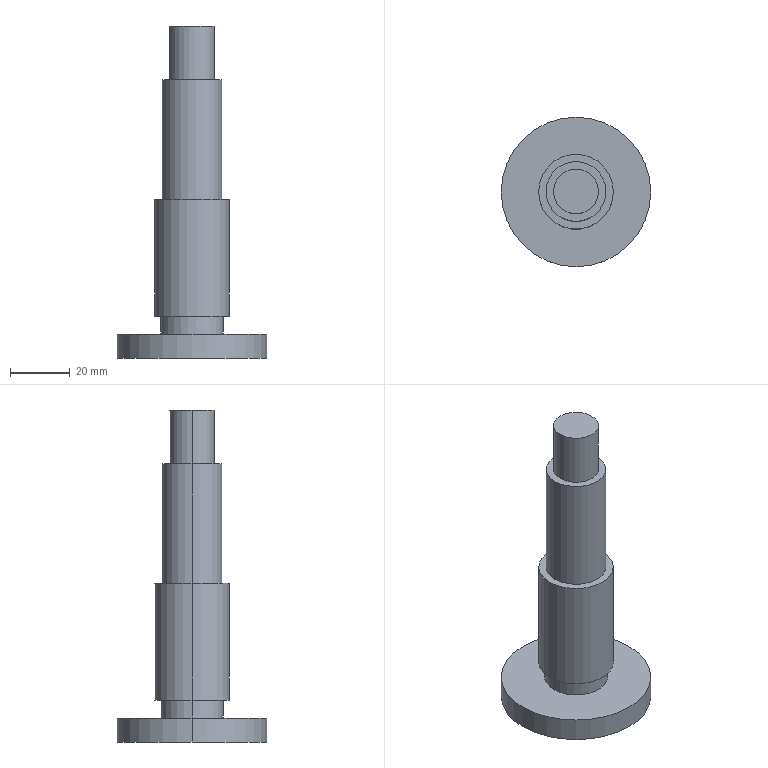Part | SolidWorks | features ICE 3, Extrusion 1, RevCut 1 | 1 solid | 16 faces | box 50 x 50 x 111 mm | volume 52677 mm3 | cylinder 10 | plane 6 | commonest cylinder face diameters 15 x2 20 x2 21 x2 25 x2 50 x2
STEP:
#1=CARTESIAN_POINT('',(7.5,0.,103.));
#2=VERTEX_POINT('',#1);
#3=CARTESIAN_POINT('',(-7.5,0.,103.));
#4=VERTEX_POINT('',#3);
#5=CARTESIAN_POINT('',(0.,0.,103.));
#6=DIRECTION('',(0.,0.,1.));
#7=DIRECTION('',(1.,0.,0.));
#8=AXIS2_PLACEMENT_3D('',#5,#6,#7);
#9=CIRCLE('',#8,7.5);
#10=EDGE_CURVE('',#2,#4,#9,.T.);
#11=ORIENTED_EDGE('',*,*,#10,.F.);
#12=CARTESIAN_POINT('',(7.5,0.,85.));
#13=VERTEX_POINT('',#12);
#14=CARTESIAN_POINT('',(7.5,0.,103.));
#15=DIRECTION('',(0.,0.,-1.));
#16=VECTOR('',#15,1000.);
#17=LINE('',#14,#16);
#18=EDGE_CURVE('',#2,#13,#17,.T.);
#19=ORIENTED_EDGE('',*,*,#18,.T.);
#20=CARTESIAN_POINT('',(-7.5,0.,85.));
#21=VERTEX_POINT('',#20);
#22=CARTESIAN_POINT('',(0.,0.,85.));
#23=DIRECTION('',(0.,0.,1.));
#24=DIRECTION('',(1.,0.,0.));
#25=AXIS2_PLACEMENT_3D('',#22,#23,#24);
#26=CIRCLE('',#25,7.5);
#27=EDGE_CURVE('',#13,#21,#26,.T.);
#28=ORIENTED_EDGE('',*,*,#27,.T.);
#29=CARTESIAN_POINT('',(-7.5,0.,103.));
#30=DIRECTION('',(0.,0.,-1.));
#31=VECTOR('',#30,1000.);
#32=LINE('',#29,#31);
#33=EDGE_CURVE('',#4,#21,#32,.T.);
#34=ORIENTED_EDGE('',*,*,#33,.F.);
#35=EDGE_LOOP('',(#11,#19,#28,#34));
#36=FACE_OUTER_BOUND('',#35,.T.);
#37=CARTESIAN_POINT('',(0.,0.,103.));
#38=DIRECTION('',(0.,0.,-1.));
#39=DIRECTION('',(-1.,0.,0.));
#40=AXIS2_PLACEMENT_3D('',#37,#38,#39);
#41=CYLINDRICAL_SURFACE('',#40,7.5);
#42=ADVANCED_FACE('',(#36),#41,.T.);
#43=CARTESIAN_POINT('',(-25.,0.,-8.));
#44=VERTEX_POINT('',#43);
#45=CARTESIAN_POINT('',(25.,0.,-8.));
#46=VERTEX_POINT('',#45);
#47=CARTESIAN_POINT('',(0.,0.,-8.));
#48=DIRECTION('',(0.,0.,-1.));
#49=DIRECTION('',(-1.,0.,0.));
#50=AXIS2_PLACEMENT_3D('',#47,#48,#49);
#51=CIRCLE('',#50,25.);
#52=EDGE_CURVE('',#44,#46,#51,.T.);
#53=ORIENTED_EDGE('',*,*,#52,.F.);
#54=CARTESIAN_POINT('',(-25.,0.,0.));
#55=VERTEX_POINT('',#54);
#56=CARTESIAN_POINT('',(-25.,0.,-8.));
#57=DIRECTION('',(0.,0.,1.));
#58=VECTOR('',#57,1000.);
#59=LINE('',#56,#58);
#60=EDGE_CURVE('',#44,#55,#59,.T.);
#61=ORIENTED_EDGE('',*,*,#60,.T.);
#62=CARTESIAN_POINT('',(25.,0.,0.));
#63=VERTEX_POINT('',#62);
#64=CARTESIAN_POINT('',(0.,0.,0.));
#65=DIRECTION('',(0.,0.,-1.));
#66=DIRECTION('',(-1.,0.,0.));
#67=AXIS2_PLACEMENT_3D('',#64,#65,#66);
#68=CIRCLE('',#67,25.);
#69=EDGE_CURVE('',#55,#63,#68,.T.);
#70=ORIENTED_EDGE('',*,*,#69,.T.);
#71=CARTESIAN_POINT('',(25.,0.,-8.));
#72=DIRECTION('',(0.,0.,1.));
#73=VECTOR('',#72,1000.);
#74=LINE('',#71,#73);
#75=EDGE_CURVE('',#46,#63,#74,.T.);
#76=ORIENTED_EDGE('',*,*,#75,.F.);
#77=EDGE_LOOP('',(#53,#61,#70,#76));
#78=FACE_OUTER_BOUND('',#77,.T.);
#79=CARTESIAN_POINT('',(0.,0.,-8.));
#80=DIRECTION('',(0.,0.,1.));
#81=DIRECTION('',(1.,0.,0.));
#82=AXIS2_PLACEMENT_3D('',#79,#80,#81);
#83=CYLINDRICAL_SURFACE('',#82,25.);
#84=ADVANCED_FACE('',(#78),#83,.T.);
#85=CARTESIAN_POINT('',(-10.5,0.,6.));
#86=VERTEX_POINT('',#85);
#87=CARTESIAN_POINT('',(10.5,0.,6.));
#88=VERTEX_POINT('',#87);
#89=CARTESIAN_POINT('',(0.,0.,6.));
#90=DIRECTION('',(0.,0.,-1.));
#91=DIRECTION('',(-1.,0.,0.));
#92=AXIS2_PLACEMENT_3D('',#89,#90,#91);
#93=CIRCLE('',#92,10.5);
#94=EDGE_CURVE('',#86,#88,#93,.T.);
#95=ORIENTED_EDGE('',*,*,#94,.T.);
#96=CARTESIAN_POINT('',(10.5,0.,0.));
#97=VERTEX_POINT('',#96);
#98=CARTESIAN_POINT('',(10.5,0.,0.));
#99=DIRECTION('',(0.,0.,-1.));
#100=VECTOR('',#99,1000.);
#101=LINE('',#98,#100);
#102=EDGE_CURVE('',#88,#97,#101,.T.);
#103=ORIENTED_EDGE('',*,*,#102,.T.);
#104=CARTESIAN_POINT('',(-10.5,0.,0.));
#105=VERTEX_POINT('',#104);
#106=CARTESIAN_POINT('',(0.,0.,0.));
#107=DIRECTION('',(0.,0.,-1.));
#108=DIRECTION('',(-1.,0.,0.));
#109=AXIS2_PLACEMENT_3D('',#106,#107,#108);
#110=CIRCLE('',#109,10.5);
#111=EDGE_CURVE('',#105,#97,#110,.T.);
#112=ORIENTED_EDGE('',*,*,#111,.F.);
#113=CARTESIAN_POINT('',(-10.5,0.,0.));
#114=DIRECTION('',(0.,0.,-1.));
#115=VECTOR('',#114,1000.);
#116=LINE('',#113,#115);
#117=EDGE_CURVE('',#86,#105,#116,.T.);
#118=ORIENTED_EDGE('',*,*,#117,.F.);
#119=EDGE_LOOP('',(#95,#103,#112,#118));
#120=FACE_OUTER_BOUND('',#119,.T.);
#121=CARTESIAN_POINT('',(0.,0.,0.));
#122=DIRECTION('',(0.,0.,-1.));
#123=DIRECTION('',(-1.,0.,0.));
#124=AXIS2_PLACEMENT_3D('',#121,#122,#123);
#125=CYLINDRICAL_SURFACE('',#124,10.5);
#126=ADVANCED_FACE('',(#120),#125,.T.);
#127=CARTESIAN_POINT('',(10.,0.,85.));
#128=VERTEX_POINT('',#127);
#129=CARTESIAN_POINT('',(-10.,0.,85.));
#130=VERTEX_POINT('',#129);
#131=CARTESIAN_POINT('',(0.,0.,85.));
#132=DIRECTION('',(0.,0.,1.));
#133=DIRECTION('',(1.,0.,0.));
#134=AXIS2_PLACEMENT_3D('',#131,#132,#133);
#135=CIRCLE('',#134,10.);
#136=EDGE_CURVE('',#128,#130,#135,.T.);
#137=ORIENTED_EDGE('',*,*,#136,.F.);
#138=CARTESIAN_POINT('',(10.,0.,45.));
#139=VERTEX_POINT('',#138);
#140=CARTESIAN_POINT('',(10.,0.,85.));
#141=DIRECTION('',(0.,0.,-1.));
#142=VECTOR('',#141,1000.);
#143=LINE('',#140,#142);
#144=EDGE_CURVE('',#128,#139,#143,.T.);
#145=ORIENTED_EDGE('',*,*,#144,.T.);
#146=CARTESIAN_POINT('',(-10.,0.,45.));
#147=VERTEX_POINT('',#146);
#148=CARTESIAN_POINT('',(0.,0.,45.));
#149=DIRECTION('',(0.,0.,1.));
#150=DIRECTION('',(1.,0.,0.));
#151=AXIS2_PLACEMENT_3D('',#148,#149,#150);
#152=CIRCLE('',#151,10.);
#153=EDGE_CURVE('',#139,#147,#152,.T.);
#154=ORIENTED_EDGE('',*,*,#153,.T.);
#155=CARTESIAN_POINT('',(-10.,0.,85.));
#156=DIRECTION('',(0.,0.,-1.));
#157=VECTOR('',#156,1000.);
#158=LINE('',#155,#157);
#159=EDGE_CURVE('',#130,#147,#158,.T.);
#160=ORIENTED_EDGE('',*,*,#159,.F.);
#161=EDGE_LOOP('',(#137,#145,#154,#160));
#162=FACE_OUTER_BOUND('',#161,.T.);
#163=CARTESIAN_POINT('',(0.,0.,85.));
#164=DIRECTION('',(0.,0.,-1.));
#165=DIRECTION('',(-1.,0.,0.));
#166=AXIS2_PLACEMENT_3D('',#163,#164,#165);
#167=CYLINDRICAL_SURFACE('',#166,10.);
#168=ADVANCED_FACE('',(#162),#167,.T.);
#169=CARTESIAN_POINT('',(12.5,0.,45.));
#170=VERTEX_POINT('',#169);
#171=CARTESIAN_POINT('',(-12.5,0.,45.));
#172=VERTEX_POINT('',#171);
#173=CARTESIAN_POINT('',(0.,0.,45.));
#174=DIRECTION('',(0.,0.,1.));
#175=DIRECTION('',(1.,0.,0.));
#176=AXIS2_PLACEMENT_3D('',#173,#174,#175);
#177=CIRCLE('',#176,12.5);
#178=EDGE_CURVE('',#170,#172,#177,.T.);
#179=ORIENTED_EDGE('',*,*,#178,.F.);
#180=CARTESIAN_POINT('',(12.5,0.,6.));
#181=VERTEX_POINT('',#180);
#182=CARTESIAN_POINT('',(12.5,0.,45.));
#183=DIRECTION('',(0.,0.,-1.));
#184=VECTOR('',#183,1000.);
#185=LINE('',#182,#184);
#186=EDGE_CURVE('',#170,#181,#185,.T.);
#187=ORIENTED_EDGE('',*,*,#186,.T.);
#188=CARTESIAN_POINT('',(-12.5,0.,6.));
#189=VERTEX_POINT('',#188);
#190=CARTESIAN_POINT('',(0.,0.,6.));
#191=DIRECTION('',(0.,0.,-1.));
#192=DIRECTION('',(-1.,0.,0.));
#193=AXIS2_PLACEMENT_3D('',#190,#191,#192);
#194=CIRCLE('',#193,12.5);
#195=EDGE_CURVE('',#189,#181,#194,.T.);
#196=ORIENTED_EDGE('',*,*,#195,.F.);
#197=CARTESIAN_POINT('',(-12.5,0.,45.));
#198=DIRECTION('',(0.,0.,-1.));
#199=VECTOR('',#198,1000.);
#200=LINE('',#197,#199);
#201=EDGE_CURVE('',#172,#189,#200,.T.);
#202=ORIENTED_EDGE('',*,*,#201,.F.);
#203=EDGE_LOOP('',(#179,#187,#196,#202));
#204=FACE_OUTER_BOUND('',#203,.T.);
#205=CARTESIAN_POINT('',(0.,0.,45.));
#206=DIRECTION('',(0.,0.,-1.));
#207=DIRECTION('',(-1.,0.,0.));
#208=AXIS2_PLACEMENT_3D('',#205,#206,#207);
#209=CYLINDRICAL_SURFACE('',#208,12.5);
#210=ADVANCED_FACE('',(#204),#209,.T.);
#211=ORIENTED_EDGE('',*,*,#186,.F.);
#212=CARTESIAN_POINT('',(0.,0.,45.));
#213=DIRECTION('',(0.,0.,1.));
#214=DIRECTION('',(1.,0.,0.));
#215=AXIS2_PLACEMENT_3D('',#212,#213,#214);
#216=CIRCLE('',#215,12.5);
#217=EDGE_CURVE('',#172,#170,#216,.T.);
#218=ORIENTED_EDGE('',*,*,#217,.F.);
#219=ORIENTED_EDGE('',*,*,#201,.T.);
#220=CARTESIAN_POINT('',(0.,0.,6.));
#221=DIRECTION('',(0.,0.,-1.));
#222=DIRECTION('',(-1.,0.,0.));
#223=AXIS2_PLACEMENT_3D('',#220,#221,#222);
#224=CIRCLE('',#223,12.5);
#225=EDGE_CURVE('',#181,#189,#224,.T.);
#226=ORIENTED_EDGE('',*,*,#225,.F.);
#227=EDGE_LOOP('',(#211,#218,#219,#226));
#228=FACE_OUTER_BOUND('',#227,.T.);
#229=CARTESIAN_POINT('',(0.,0.,45.));
#230=DIRECTION('',(0.,0.,-1.));
#231=DIRECTION('',(-1.,0.,0.));
#232=AXIS2_PLACEMENT_3D('',#229,#230,#231);
#233=CYLINDRICAL_SURFACE('',#232,12.5);
#234=ADVANCED_FACE('',(#228),#233,.T.);
#235=CARTESIAN_POINT('',(0.,0.,45.));
#236=DIRECTION('',(0.,0.,1.));
#237=DIRECTION('',(1.,0.,0.));
#238=AXIS2_PLACEMENT_3D('',#235,#236,#237);
#239=CIRCLE('',#238,10.);
#240=EDGE_CURVE('',#147,#139,#239,.T.);
#241=ORIENTED_EDGE('',*,*,#240,.F.);
#242=ORIENTED_EDGE('',*,*,#153,.F.);
#243=EDGE_LOOP('',(#241,#242));
#244=FACE_BOUND('',#243,.T.);
#245=ORIENTED_EDGE('',*,*,#217,.T.);
#246=ORIENTED_EDGE('',*,*,#178,.T.);
#247=EDGE_LOOP('',(#245,#246));
#248=FACE_OUTER_BOUND('',#247,.T.);
#249=CARTESIAN_POINT('',(0.,0.,45.));
#250=DIRECTION('',(0.,0.,1.));
#251=DIRECTION('',(1.,0.,0.));
#252=AXIS2_PLACEMENT_3D('',#249,#250,#251);
#253=PLANE('',#252);
#254=ADVANCED_FACE('',(#244,#248),#253,.T.);
#255=ORIENTED_EDGE('',*,*,#144,.F.);
#256=CARTESIAN_POINT('',(0.,0.,85.));
#257=DIRECTION('',(0.,0.,1.));
#258=DIRECTION('',(1.,0.,0.));
#259=AXIS2_PLACEMENT_3D('',#256,#257,#258);
#260=CIRCLE('',#259,10.);
#261=EDGE_CURVE('',#130,#128,#260,.T.);
#262=ORIENTED_EDGE('',*,*,#261,.F.);
#263=ORIENTED_EDGE('',*,*,#159,.T.);
#264=ORIENTED_EDGE('',*,*,#240,.T.);
#265=EDGE_LOOP('',(#255,#262,#263,#264));
#266=FACE_OUTER_BOUND('',#265,.T.);
#267=CARTESIAN_POINT('',(0.,0.,85.));
#268=DIRECTION('',(0.,0.,-1.));
#269=DIRECTION('',(-1.,0.,0.));
#270=AXIS2_PLACEMENT_3D('',#267,#268,#269);
#271=CYLINDRICAL_SURFACE('',#270,10.);
#272=ADVANCED_FACE('',(#266),#271,.T.);
#273=CARTESIAN_POINT('',(0.,0.,85.));
#274=DIRECTION('',(0.,0.,1.));
#275=DIRECTION('',(1.,0.,0.));
#276=AXIS2_PLACEMENT_3D('',#273,#274,#275);
#277=CIRCLE('',#276,7.5);
#278=EDGE_CURVE('',#21,#13,#277,.T.);
#279=ORIENTED_EDGE('',*,*,#278,.F.);
#280=ORIENTED_EDGE('',*,*,#27,.F.);
#281=EDGE_LOOP('',(#279,#280));
#282=FACE_BOUND('',#281,.T.);
#283=ORIENTED_EDGE('',*,*,#261,.T.);
#284=ORIENTED_EDGE('',*,*,#136,.T.);
#285=EDGE_LOOP('',(#283,#284));
#286=FACE_OUTER_BOUND('',#285,.T.);
#287=CARTESIAN_POINT('',(0.,0.,85.));
#288=DIRECTION('',(0.,0.,1.));
#289=DIRECTION('',(1.,0.,0.));
#290=AXIS2_PLACEMENT_3D('',#287,#288,#289);
#291=PLANE('',#290);
#292=ADVANCED_FACE('',(#282,#286),#291,.T.);
#293=ORIENTED_EDGE('',*,*,#102,.F.);
#294=CARTESIAN_POINT('',(0.,0.,6.));
#295=DIRECTION('',(0.,0.,-1.));
#296=DIRECTION('',(-1.,0.,0.));
#297=AXIS2_PLACEMENT_3D('',#294,#295,#296);
#298=CIRCLE('',#297,10.5);
#299=EDGE_CURVE('',#88,#86,#298,.T.);
#300=ORIENTED_EDGE('',*,*,#299,.T.);
#301=ORIENTED_EDGE('',*,*,#117,.T.);
#302=CARTESIAN_POINT('',(0.,0.,0.));
#303=DIRECTION('',(0.,0.,-1.));
#304=DIRECTION('',(-1.,0.,0.));
#305=AXIS2_PLACEMENT_3D('',#302,#303,#304);
#306=CIRCLE('',#305,10.5);
#307=EDGE_CURVE('',#97,#105,#306,.T.);
#308=ORIENTED_EDGE('',*,*,#307,.F.);
#309=EDGE_LOOP('',(#293,#300,#301,#308));
#310=FACE_OUTER_BOUND('',#309,.T.);
#311=CARTESIAN_POINT('',(0.,0.,0.));
#312=DIRECTION('',(0.,0.,-1.));
#313=DIRECTION('',(-1.,0.,0.));
#314=AXIS2_PLACEMENT_3D('',#311,#312,#313);
#315=CYLINDRICAL_SURFACE('',#314,10.5);
#316=ADVANCED_FACE('',(#310),#315,.T.);
#317=ORIENTED_EDGE('',*,*,#195,.T.);
#318=ORIENTED_EDGE('',*,*,#225,.T.);
#319=EDGE_LOOP('',(#317,#318));
#320=FACE_OUTER_BOUND('',#319,.T.);
#321=ORIENTED_EDGE('',*,*,#94,.F.);
#322=ORIENTED_EDGE('',*,*,#299,.F.);
#323=EDGE_LOOP('',(#321,#322));
#324=FACE_BOUND('',#323,.T.);
#325=CARTESIAN_POINT('',(10.5,0.,6.));
#326=DIRECTION('',(0.,0.,-1.));
#327=DIRECTION('',(-1.,0.,0.));
#328=AXIS2_PLACEMENT_3D('',#325,#326,#327);
#329=PLANE('',#328);
#330=ADVANCED_FACE('',(#320,#324),#329,.T.);
#331=CARTESIAN_POINT('',(0.,0.,-8.));
#332=DIRECTION('',(0.,0.,-1.));
#333=DIRECTION('',(-1.,0.,0.));
#334=AXIS2_PLACEMENT_3D('',#331,#332,#333);
#335=CIRCLE('',#334,25.);
#336=EDGE_CURVE('',#46,#44,#335,.T.);
#337=ORIENTED_EDGE('',*,*,#336,.T.);
#338=ORIENTED_EDGE('',*,*,#52,.T.);
#339=EDGE_LOOP('',(#337,#338));
#340=FACE_OUTER_BOUND('',#339,.T.);
#341=CARTESIAN_POINT('',(0.,0.,-8.));
#342=DIRECTION('',(0.,0.,-1.));
#343=DIRECTION('',(-1.,0.,0.));
#344=AXIS2_PLACEMENT_3D('',#341,#342,#343);
#345=PLANE('',#344);
#346=ADVANCED_FACE('',(#340),#345,.T.);
#347=ORIENTED_EDGE('',*,*,#60,.F.);
#348=ORIENTED_EDGE('',*,*,#336,.F.);
#349=ORIENTED_EDGE('',*,*,#75,.T.);
#350=CARTESIAN_POINT('',(0.,0.,0.));
#351=DIRECTION('',(0.,0.,-1.));
#352=DIRECTION('',(-1.,0.,0.));
#353=AXIS2_PLACEMENT_3D('',#350,#351,#352);
#354=CIRCLE('',#353,25.);
#355=EDGE_CURVE('',#63,#55,#354,.T.);
#356=ORIENTED_EDGE('',*,*,#355,.T.);
#357=EDGE_LOOP('',(#347,#348,#349,#356));
#358=FACE_OUTER_BOUND('',#357,.T.);
#359=CARTESIAN_POINT('',(0.,0.,-8.));
#360=DIRECTION('',(0.,0.,1.));
#361=DIRECTION('',(1.,0.,0.));
#362=AXIS2_PLACEMENT_3D('',#359,#360,#361);
#363=CYLINDRICAL_SURFACE('',#362,25.);
#364=ADVANCED_FACE('',(#358),#363,.T.);
#365=ORIENTED_EDGE('',*,*,#355,.F.);
#366=ORIENTED_EDGE('',*,*,#69,.F.);
#367=EDGE_LOOP('',(#365,#366));
#368=FACE_OUTER_BOUND('',#367,.T.);
#369=ORIENTED_EDGE('',*,*,#111,.T.);
#370=ORIENTED_EDGE('',*,*,#307,.T.);
#371=EDGE_LOOP('',(#369,#370));
#372=FACE_BOUND('',#371,.T.);
#373=CARTESIAN_POINT('',(0.,0.,0.));
#374=DIRECTION('',(0.,0.,-1.));
#375=DIRECTION('',(-1.,0.,0.));
#376=AXIS2_PLACEMENT_3D('',#373,#374,#375);
#377=PLANE('',#376);
#378=ADVANCED_FACE('',(#368,#372),#377,.F.);
#379=ORIENTED_EDGE('',*,*,#18,.F.);
#380=CARTESIAN_POINT('',(0.,0.,103.));
#381=DIRECTION('',(0.,0.,1.));
#382=DIRECTION('',(1.,0.,0.));
#383=AXIS2_PLACEMENT_3D('',#380,#381,#382);
#384=CIRCLE('',#383,7.5);
#385=EDGE_CURVE('',#4,#2,#384,.T.);
#386=ORIENTED_EDGE('',*,*,#385,.F.);
#387=ORIENTED_EDGE('',*,*,#33,.T.);
#388=ORIENTED_EDGE('',*,*,#278,.T.);
#389=EDGE_LOOP('',(#379,#386,#387,#388));
#390=FACE_OUTER_BOUND('',#389,.T.);
#391=CARTESIAN_POINT('',(0.,0.,103.));
#392=DIRECTION('',(0.,0.,-1.));
#393=DIRECTION('',(-1.,0.,0.));
#394=AXIS2_PLACEMENT_3D('',#391,#392,#393);
#395=CYLINDRICAL_SURFACE('',#394,7.5);
#396=ADVANCED_FACE('',(#390),#395,.T.);
#397=ORIENTED_EDGE('',*,*,#385,.T.);
#398=ORIENTED_EDGE('',*,*,#10,.T.);
#399=EDGE_LOOP('',(#397,#398));
#400=FACE_OUTER_BOUND('',#399,.T.);
#401=CARTESIAN_POINT('',(0.,0.,103.));
#402=DIRECTION('',(0.,0.,1.));
#403=DIRECTION('',(1.,0.,0.));
#404=AXIS2_PLACEMENT_3D('',#401,#402,#403);
#405=PLANE('',#404);
#406=ADVANCED_FACE('',(#400),#405,.T.);
#407=CLOSED_SHELL('',(#42,#84,#126,#168,#210,#234,#254,#272,#292,#316,#330,#346,#364,#378,#396,#406));
#408=MANIFOLD_SOLID_BREP('',#407);
#409=CARTESIAN_POINT('',(0.,0.,0.));
#410=DIRECTION('',(0.,0.,1.));
#411=DIRECTION('',(1.,0.,0.));
#412=AXIS2_PLACEMENT_3D('',#409,#410,#411);
#413=(LENGTH_UNIT()NAMED_UNIT(*)SI_UNIT(.MILLI.,.METRE.));
#414=UNCERTAINTY_MEASURE_WITH_UNIT(LENGTH_MEASURE(0.00001),#413,'','');
#415=(NAMED_UNIT(*)PLANE_ANGLE_UNIT()SI_UNIT($,.RADIAN.));
#416=(NAMED_UNIT(*)SI_UNIT($,.STERADIAN.)SOLID_ANGLE_UNIT());
#417=(GEOMETRIC_REPRESENTATION_CONTEXT(3)GLOBAL_UNCERTAINTY_ASSIGNED_CONTEXT((#414))GLOBAL_UNIT_ASSIGNED_CONTEXT((#413,#415,#416))REPRESENTATION_CONTEXT('',''));
#418=ADVANCED_BREP_SHAPE_REPRESENTATION('',(#408,#412),#417);